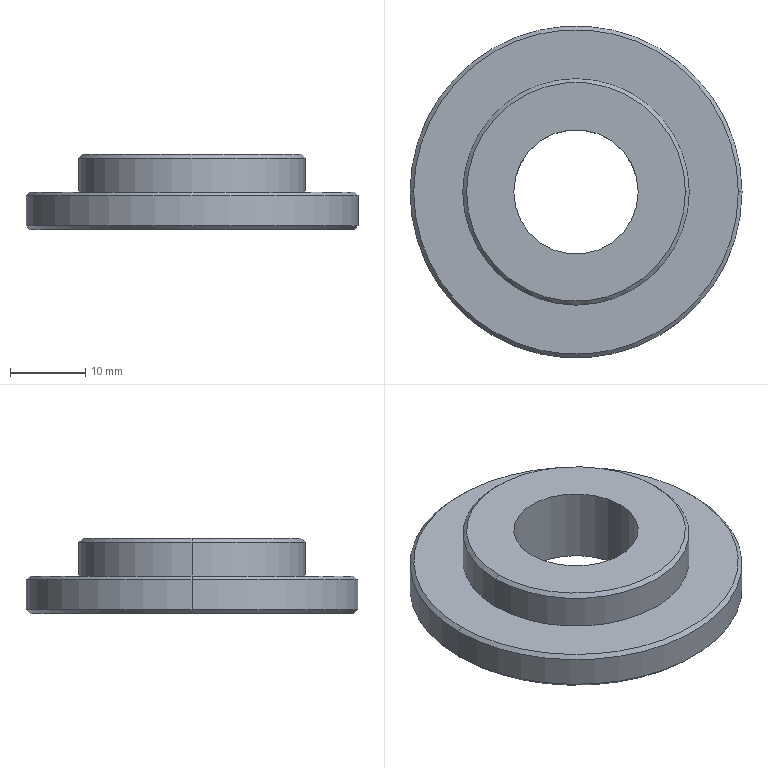Part | STEP file | 2025 Spring plate | 1 solid | 15 faces | box 44 x 44 x 10 mm | volume 8953 mm3 | cone 6 | cylinder 6 | plane 3 | commonest cylinder face diameters 16.5 x2 30 x2 44 x2
STEP:
#1=CARTESIAN_POINT('',(0.,0.,0.));
#2=DIRECTION('',(0.,0.,1.));
#3=DIRECTION('',(1.,0.,0.));
#4=AXIS2_PLACEMENT_3D('',#1,#2,#3);
#5=CARTESIAN_POINT('',(14.5,0.,10.));
#6=VERTEX_POINT('',#5);
#7=CARTESIAN_POINT('',(-14.5,0.,10.));
#8=VERTEX_POINT('',#7);
#9=CARTESIAN_POINT('',(0.,0.,10.));
#10=DIRECTION('',(0.,0.,1.));
#11=DIRECTION('',(1.,0.,0.));
#12=AXIS2_PLACEMENT_3D('',#9,#10,#11);
#13=CIRCLE('',#12,14.5);
#14=CARTESIAN_POINT('',(0.,0.,10.));
#15=DIRECTION('',(0.,0.,-1.));
#16=DIRECTION('',(-1.,0.,0.));
#17=AXIS2_PLACEMENT_3D('',#14,#15,#16);
#18=CONICAL_SURFACE('',#17,14.5,0.7854);
#19=CARTESIAN_POINT('',(3.142,0.));
#20=DIRECTION('',(-1.,0.));
#21=VECTOR('',#20,1.);
#22=LINE('',#19,#21);
#23=(GEOMETRIC_REPRESENTATION_CONTEXT(2)PARAMETRIC_REPRESENTATION_CONTEXT()REPRESENTATION_CONTEXT('',''));
#24=DEFINITIONAL_REPRESENTATION('',(#22),#23);
#25=PCURVE('',#18,#24);
#26=CARTESIAN_POINT('',(0.,0.,10.));
#27=DIRECTION('',(0.,0.,1.));
#28=DIRECTION('',(1.,0.,0.));
#29=AXIS2_PLACEMENT_3D('',#26,#27,#28);
#30=PLANE('',#29);
#31=CARTESIAN_POINT('',(0.,0.));
#32=DIRECTION('',(1.,0.));
#33=AXIS2_PLACEMENT_2D('',#31,#32);
#34=CIRCLE('',#33,14.5);
#35=(GEOMETRIC_REPRESENTATION_CONTEXT(2)PARAMETRIC_REPRESENTATION_CONTEXT()REPRESENTATION_CONTEXT('',''));
#36=DEFINITIONAL_REPRESENTATION('',(#34),#35);
#37=PCURVE('',#30,#36);
#38=SURFACE_CURVE('',#13,(#25,#37),.PCURVE_S1.);
#39=EDGE_CURVE('',#6,#8,#38,.T.);
#40=ORIENTED_EDGE('',*,*,#39,.F.);
#41=CARTESIAN_POINT('',(15.,0.,9.5));
#42=VERTEX_POINT('',#41);
#43=CARTESIAN_POINT('',(14.5,0.,10.));
#44=DIRECTION('',(0.7071,0.,-0.7071));
#45=VECTOR('',#44,1.);
#46=LINE('',#43,#45);
#47=CARTESIAN_POINT('',(3.142,0.));
#48=DIRECTION('',(0.,1.));
#49=VECTOR('',#48,1.);
#50=LINE('',#47,#49);
#51=(GEOMETRIC_REPRESENTATION_CONTEXT(2)PARAMETRIC_REPRESENTATION_CONTEXT()REPRESENTATION_CONTEXT('',''));
#52=DEFINITIONAL_REPRESENTATION('',(#50),#51);
#53=PCURVE('',#18,#52);
#54=CARTESIAN_POINT('',(0.,0.,10.));
#55=DIRECTION('',(0.,0.,-1.));
#56=DIRECTION('',(-1.,0.,0.));
#57=AXIS2_PLACEMENT_3D('',#54,#55,#56);
#58=CONICAL_SURFACE('',#57,14.5,0.7854);
#59=CARTESIAN_POINT('',(3.142,0.));
#60=DIRECTION('',(0.,1.));
#61=VECTOR('',#60,1.);
#62=LINE('',#59,#61);
#63=(GEOMETRIC_REPRESENTATION_CONTEXT(2)PARAMETRIC_REPRESENTATION_CONTEXT()REPRESENTATION_CONTEXT('',''));
#64=DEFINITIONAL_REPRESENTATION('',(#62),#63);
#65=PCURVE('',#58,#64);
#66=SURFACE_CURVE('',#46,(#53,#65),.PCURVE_S1.);
#67=EDGE_CURVE('',#6,#42,#66,.T.);
#68=ORIENTED_EDGE('',*,*,#67,.T.);
#69=CARTESIAN_POINT('',(-15.,0.,9.5));
#70=VERTEX_POINT('',#69);
#71=CARTESIAN_POINT('',(0.,0.,9.5));
#72=DIRECTION('',(0.,0.,-1.));
#73=DIRECTION('',(1.,0.,0.));
#74=AXIS2_PLACEMENT_3D('',#71,#72,#73);
#75=CIRCLE('',#74,15.);
#76=CARTESIAN_POINT('',(-3.142,0.5));
#77=DIRECTION('',(1.,0.));
#78=VECTOR('',#77,1.);
#79=LINE('',#76,#78);
#80=(GEOMETRIC_REPRESENTATION_CONTEXT(2)PARAMETRIC_REPRESENTATION_CONTEXT()REPRESENTATION_CONTEXT('',''));
#81=DEFINITIONAL_REPRESENTATION('',(#79),#80);
#82=PCURVE('',#18,#81);
#83=CARTESIAN_POINT('',(0.,0.,10.));
#84=DIRECTION('',(0.,0.,-1.));
#85=DIRECTION('',(-1.,0.,0.));
#86=AXIS2_PLACEMENT_3D('',#83,#84,#85);
#87=CYLINDRICAL_SURFACE('',#86,15.);
#88=CARTESIAN_POINT('',(-3.142,0.5));
#89=DIRECTION('',(1.,0.));
#90=VECTOR('',#89,1.);
#91=LINE('',#88,#90);
#92=(GEOMETRIC_REPRESENTATION_CONTEXT(2)PARAMETRIC_REPRESENTATION_CONTEXT()REPRESENTATION_CONTEXT('',''));
#93=DEFINITIONAL_REPRESENTATION('',(#91),#92);
#94=PCURVE('',#87,#93);
#95=SURFACE_CURVE('',#75,(#82,#94),.PCURVE_S1.);
#96=EDGE_CURVE('',#70,#42,#95,.T.);
#97=ORIENTED_EDGE('',*,*,#96,.F.);
#98=CARTESIAN_POINT('',(-14.5,0.,10.));
#99=DIRECTION('',(-0.7071,0.,-0.7071));
#100=VECTOR('',#99,1.);
#101=LINE('',#98,#100);
#102=CARTESIAN_POINT('',(0.,0.));
#103=DIRECTION('',(0.,1.));
#104=VECTOR('',#103,1.);
#105=LINE('',#102,#104);
#106=(GEOMETRIC_REPRESENTATION_CONTEXT(2)PARAMETRIC_REPRESENTATION_CONTEXT()REPRESENTATION_CONTEXT('',''));
#107=DEFINITIONAL_REPRESENTATION('',(#105),#106);
#108=PCURVE('',#18,#107);
#109=CARTESIAN_POINT('',(6.283,0.));
#110=DIRECTION('',(0.,1.));
#111=VECTOR('',#110,1.);
#112=LINE('',#109,#111);
#113=(GEOMETRIC_REPRESENTATION_CONTEXT(2)PARAMETRIC_REPRESENTATION_CONTEXT()REPRESENTATION_CONTEXT('',''));
#114=DEFINITIONAL_REPRESENTATION('',(#112),#113);
#115=PCURVE('',#58,#114);
#116=SURFACE_CURVE('',#101,(#108,#115),.PCURVE_S1.);
#117=EDGE_CURVE('',#8,#70,#116,.T.);
#118=ORIENTED_EDGE('',*,*,#117,.F.);
#119=EDGE_LOOP('',(#40,#68,#97,#118));
#120=FACE_BOUND('',#119,.T.);
#121=ADVANCED_FACE('',(#120),#18,.T.);
#122=CARTESIAN_POINT('',(21.5,0.,5.));
#123=VERTEX_POINT('',#122);
#124=CARTESIAN_POINT('',(-21.5,0.,5.));
#125=VERTEX_POINT('',#124);
#126=CARTESIAN_POINT('',(0.,0.,5.));
#127=DIRECTION('',(0.,0.,1.));
#128=DIRECTION('',(1.,0.,0.));
#129=AXIS2_PLACEMENT_3D('',#126,#127,#128);
#130=CIRCLE('',#129,21.5);
#131=CARTESIAN_POINT('',(0.,0.,5.));
#132=DIRECTION('',(0.,0.,-1.));
#133=DIRECTION('',(-1.,0.,0.));
#134=AXIS2_PLACEMENT_3D('',#131,#132,#133);
#135=CONICAL_SURFACE('',#134,21.5,0.7854);
#136=CARTESIAN_POINT('',(3.142,0.));
#137=DIRECTION('',(-1.,0.));
#138=VECTOR('',#137,1.);
#139=LINE('',#136,#138);
#140=(GEOMETRIC_REPRESENTATION_CONTEXT(2)PARAMETRIC_REPRESENTATION_CONTEXT()REPRESENTATION_CONTEXT('',''));
#141=DEFINITIONAL_REPRESENTATION('',(#139),#140);
#142=PCURVE('',#135,#141);
#143=CARTESIAN_POINT('',(0.,0.,5.));
#144=DIRECTION('',(0.,0.,1.));
#145=DIRECTION('',(1.,0.,0.));
#146=AXIS2_PLACEMENT_3D('',#143,#144,#145);
#147=PLANE('',#146);
#148=CARTESIAN_POINT('',(0.,0.));
#149=DIRECTION('',(1.,0.));
#150=AXIS2_PLACEMENT_2D('',#148,#149);
#151=CIRCLE('',#150,21.5);
#152=(GEOMETRIC_REPRESENTATION_CONTEXT(2)PARAMETRIC_REPRESENTATION_CONTEXT()REPRESENTATION_CONTEXT('',''));
#153=DEFINITIONAL_REPRESENTATION('',(#151),#152);
#154=PCURVE('',#147,#153);
#155=SURFACE_CURVE('',#130,(#142,#154),.PCURVE_S1.);
#156=EDGE_CURVE('',#123,#125,#155,.T.);
#157=ORIENTED_EDGE('',*,*,#156,.F.);
#158=CARTESIAN_POINT('',(22.,0.,4.5));
#159=VERTEX_POINT('',#158);
#160=CARTESIAN_POINT('',(21.5,0.,5.));
#161=DIRECTION('',(0.7071,0.,-0.7071));
#162=VECTOR('',#161,1.);
#163=LINE('',#160,#162);
#164=CARTESIAN_POINT('',(3.142,0.));
#165=DIRECTION('',(0.,1.));
#166=VECTOR('',#165,1.);
#167=LINE('',#164,#166);
#168=(GEOMETRIC_REPRESENTATION_CONTEXT(2)PARAMETRIC_REPRESENTATION_CONTEXT()REPRESENTATION_CONTEXT('',''));
#169=DEFINITIONAL_REPRESENTATION('',(#167),#168);
#170=PCURVE('',#135,#169);
#171=CARTESIAN_POINT('',(0.,0.,5.));
#172=DIRECTION('',(0.,0.,-1.));
#173=DIRECTION('',(-1.,0.,0.));
#174=AXIS2_PLACEMENT_3D('',#171,#172,#173);
#175=CONICAL_SURFACE('',#174,21.5,0.7854);
#176=CARTESIAN_POINT('',(3.142,0.));
#177=DIRECTION('',(0.,1.));
#178=VECTOR('',#177,1.);
#179=LINE('',#176,#178);
#180=(GEOMETRIC_REPRESENTATION_CONTEXT(2)PARAMETRIC_REPRESENTATION_CONTEXT()REPRESENTATION_CONTEXT('',''));
#181=DEFINITIONAL_REPRESENTATION('',(#179),#180);
#182=PCURVE('',#175,#181);
#183=SURFACE_CURVE('',#163,(#170,#182),.PCURVE_S1.);
#184=EDGE_CURVE('',#123,#159,#183,.T.);
#185=ORIENTED_EDGE('',*,*,#184,.T.);
#186=CARTESIAN_POINT('',(-22.,0.,4.5));
#187=VERTEX_POINT('',#186);
#188=CARTESIAN_POINT('',(0.,0.,4.5));
#189=DIRECTION('',(0.,0.,-1.));
#190=DIRECTION('',(1.,0.,0.));
#191=AXIS2_PLACEMENT_3D('',#188,#189,#190);
#192=CIRCLE('',#191,22.);
#193=CARTESIAN_POINT('',(-3.142,0.5));
#194=DIRECTION('',(1.,0.));
#195=VECTOR('',#194,1.);
#196=LINE('',#193,#195);
#197=(GEOMETRIC_REPRESENTATION_CONTEXT(2)PARAMETRIC_REPRESENTATION_CONTEXT()REPRESENTATION_CONTEXT('',''));
#198=DEFINITIONAL_REPRESENTATION('',(#196),#197);
#199=PCURVE('',#135,#198);
#200=CARTESIAN_POINT('',(0.,0.,5.));
#201=DIRECTION('',(0.,0.,-1.));
#202=DIRECTION('',(-1.,0.,0.));
#203=AXIS2_PLACEMENT_3D('',#200,#201,#202);
#204=CYLINDRICAL_SURFACE('',#203,22.);
#205=CARTESIAN_POINT('',(-3.142,0.5));
#206=DIRECTION('',(1.,0.));
#207=VECTOR('',#206,1.);
#208=LINE('',#205,#207);
#209=(GEOMETRIC_REPRESENTATION_CONTEXT(2)PARAMETRIC_REPRESENTATION_CONTEXT()REPRESENTATION_CONTEXT('',''));
#210=DEFINITIONAL_REPRESENTATION('',(#208),#209);
#211=PCURVE('',#204,#210);
#212=SURFACE_CURVE('',#192,(#199,#211),.PCURVE_S1.);
#213=EDGE_CURVE('',#187,#159,#212,.T.);
#214=ORIENTED_EDGE('',*,*,#213,.F.);
#215=CARTESIAN_POINT('',(-21.5,0.,5.));
#216=DIRECTION('',(-0.7071,0.,-0.7071));
#217=VECTOR('',#216,1.);
#218=LINE('',#215,#217);
#219=CARTESIAN_POINT('',(0.,0.));
#220=DIRECTION('',(0.,1.));
#221=VECTOR('',#220,1.);
#222=LINE('',#219,#221);
#223=(GEOMETRIC_REPRESENTATION_CONTEXT(2)PARAMETRIC_REPRESENTATION_CONTEXT()REPRESENTATION_CONTEXT('',''));
#224=DEFINITIONAL_REPRESENTATION('',(#222),#223);
#225=PCURVE('',#135,#224);
#226=CARTESIAN_POINT('',(6.283,0.));
#227=DIRECTION('',(0.,1.));
#228=VECTOR('',#227,1.);
#229=LINE('',#226,#228);
#230=(GEOMETRIC_REPRESENTATION_CONTEXT(2)PARAMETRIC_REPRESENTATION_CONTEXT()REPRESENTATION_CONTEXT('',''));
#231=DEFINITIONAL_REPRESENTATION('',(#229),#230);
#232=PCURVE('',#175,#231);
#233=SURFACE_CURVE('',#218,(#225,#232),.PCURVE_S1.);
#234=EDGE_CURVE('',#125,#187,#233,.T.);
#235=ORIENTED_EDGE('',*,*,#234,.F.);
#236=EDGE_LOOP('',(#157,#185,#214,#235));
#237=FACE_BOUND('',#236,.T.);
#238=ADVANCED_FACE('',(#237),#135,.T.);
#239=CARTESIAN_POINT('',(-21.5,0.,0.));
#240=VERTEX_POINT('',#239);
#241=CARTESIAN_POINT('',(21.5,0.,0.));
#242=VERTEX_POINT('',#241);
#243=CARTESIAN_POINT('',(0.,0.,0.));
#244=DIRECTION('',(0.,0.,-1.));
#245=DIRECTION('',(1.,0.,0.));
#246=AXIS2_PLACEMENT_3D('',#243,#244,#245);
#247=CIRCLE('',#246,21.5);
#248=CARTESIAN_POINT('',(0.,0.,0.5));
#249=DIRECTION('',(0.,0.,1.));
#250=DIRECTION('',(1.,0.,0.));
#251=AXIS2_PLACEMENT_3D('',#248,#249,#250);
#252=CONICAL_SURFACE('',#251,22.,0.7854);
#253=CARTESIAN_POINT('',(6.283,-0.5));
#254=DIRECTION('',(-1.,0.));
#255=VECTOR('',#254,1.);
#256=LINE('',#253,#255);
#257=(GEOMETRIC_REPRESENTATION_CONTEXT(2)PARAMETRIC_REPRESENTATION_CONTEXT()REPRESENTATION_CONTEXT('',''));
#258=DEFINITIONAL_REPRESENTATION('',(#256),#257);
#259=PCURVE('',#252,#258);
#260=CARTESIAN_POINT('',(0.,0.,0.));
#261=DIRECTION('',(0.,0.,1.));
#262=DIRECTION('',(1.,0.,0.));
#263=AXIS2_PLACEMENT_3D('',#260,#261,#262);
#264=PLANE('',#263);
#265=CARTESIAN_POINT('',(21.5,0.));
#266=CARTESIAN_POINT('',(21.5,-37.239));
#267=CARTESIAN_POINT('',(-10.75,-18.62));
#268=CARTESIAN_POINT('',(-43.,0.));
#269=CARTESIAN_POINT('',(-10.75,18.62));
#270=CARTESIAN_POINT('',(21.5,37.239));
#271=CARTESIAN_POINT('',(21.5,0.));
#272=(BOUNDED_CURVE()B_SPLINE_CURVE(2,(#265,#266,#267,#268,#269,#270,#271),.UNSPECIFIED.,.T.,.F.)B_SPLINE_CURVE_WITH_KNOTS((1,2,2,2,2,1),(-2.094,0.,2.094,4.189,6.283,8.378),.UNSPECIFIED.)CURVE()GEOMETRIC_REPRESENTATION_ITEM()RATIONAL_B_SPLINE_CURVE((1.,0.5,1.,0.5,1.,0.5,1.))REPRESENTATION_ITEM(''));
#273=(GEOMETRIC_REPRESENTATION_CONTEXT(2)PARAMETRIC_REPRESENTATION_CONTEXT()REPRESENTATION_CONTEXT('',''));
#274=DEFINITIONAL_REPRESENTATION('',(#272),#273);
#275=PCURVE('',#264,#274);
#276=SURFACE_CURVE('',#247,(#259,#275),.PCURVE_S1.);
#277=EDGE_CURVE('',#240,#242,#276,.T.);
#278=ORIENTED_EDGE('',*,*,#277,.F.);
#279=CARTESIAN_POINT('',(-22.,0.,0.5));
#280=VERTEX_POINT('',#279);
#281=CARTESIAN_POINT('',(-22.,0.,0.5));
#282=DIRECTION('',(-0.7071,0.,0.7071));
#283=VECTOR('',#282,1.);
#284=LINE('',#281,#283);
#285=CARTESIAN_POINT('',(3.142,0.));
#286=DIRECTION('',(0.,1.));
#287=VECTOR('',#286,1.);
#288=LINE('',#285,#287);
#289=(GEOMETRIC_REPRESENTATION_CONTEXT(2)PARAMETRIC_REPRESENTATION_CONTEXT()REPRESENTATION_CONTEXT('',''));
#290=DEFINITIONAL_REPRESENTATION('',(#288),#289);
#291=PCURVE('',#252,#290);
#292=CARTESIAN_POINT('',(0.,0.,0.5));
#293=DIRECTION('',(0.,0.,1.));
#294=DIRECTION('',(1.,0.,0.));
#295=AXIS2_PLACEMENT_3D('',#292,#293,#294);
#296=CONICAL_SURFACE('',#295,22.,0.7854);
#297=CARTESIAN_POINT('',(3.142,0.));
#298=DIRECTION('',(0.,1.));
#299=VECTOR('',#298,1.);
#300=LINE('',#297,#299);
#301=(GEOMETRIC_REPRESENTATION_CONTEXT(2)PARAMETRIC_REPRESENTATION_CONTEXT()REPRESENTATION_CONTEXT('',''));
#302=DEFINITIONAL_REPRESENTATION('',(#300),#301);
#303=PCURVE('',#296,#302);
#304=SURFACE_CURVE('',#284,(#291,#303),.PCURVE_S1.);
#305=EDGE_CURVE('',#240,#280,#304,.T.);
#306=ORIENTED_EDGE('',*,*,#305,.T.);
#307=CARTESIAN_POINT('',(22.,0.,0.5));
#308=VERTEX_POINT('',#307);
#309=CARTESIAN_POINT('',(0.,0.,0.5));
#310=DIRECTION('',(0.,0.,1.));
#311=DIRECTION('',(1.,0.,0.));
#312=AXIS2_PLACEMENT_3D('',#309,#310,#311);
#313=CIRCLE('',#312,22.);
#314=CARTESIAN_POINT('',(0.,0.));
#315=DIRECTION('',(1.,0.));
#316=VECTOR('',#315,1.);
#317=LINE('',#314,#316);
#318=(GEOMETRIC_REPRESENTATION_CONTEXT(2)PARAMETRIC_REPRESENTATION_CONTEXT()REPRESENTATION_CONTEXT('',''));
#319=DEFINITIONAL_REPRESENTATION('',(#317),#318);
#320=PCURVE('',#252,#319);
#321=CARTESIAN_POINT('',(3.142,4.5));
#322=DIRECTION('',(-1.,0.));
#323=VECTOR('',#322,1.);
#324=LINE('',#321,#323);
#325=(GEOMETRIC_REPRESENTATION_CONTEXT(2)PARAMETRIC_REPRESENTATION_CONTEXT()REPRESENTATION_CONTEXT('',''));
#326=DEFINITIONAL_REPRESENTATION('',(#324),#325);
#327=PCURVE('',#204,#326);
#328=SURFACE_CURVE('',#313,(#320,#327),.PCURVE_S1.);
#329=EDGE_CURVE('',#308,#280,#328,.T.);
#330=ORIENTED_EDGE('',*,*,#329,.F.);
#331=CARTESIAN_POINT('',(22.,0.,0.5));
#332=DIRECTION('',(0.7071,0.,0.7071));
#333=VECTOR('',#332,1.);
#334=LINE('',#331,#333);
#335=CARTESIAN_POINT('',(0.,0.));
#336=DIRECTION('',(0.,1.));
#337=VECTOR('',#336,1.);
#338=LINE('',#335,#337);
#339=(GEOMETRIC_REPRESENTATION_CONTEXT(2)PARAMETRIC_REPRESENTATION_CONTEXT()REPRESENTATION_CONTEXT('',''));
#340=DEFINITIONAL_REPRESENTATION('',(#338),#339);
#341=PCURVE('',#252,#340);
#342=CARTESIAN_POINT('',(6.283,0.));
#343=DIRECTION('',(0.,1.));
#344=VECTOR('',#343,1.);
#345=LINE('',#342,#344);
#346=(GEOMETRIC_REPRESENTATION_CONTEXT(2)PARAMETRIC_REPRESENTATION_CONTEXT()REPRESENTATION_CONTEXT('',''));
#347=DEFINITIONAL_REPRESENTATION('',(#345),#346);
#348=PCURVE('',#296,#347);
#349=SURFACE_CURVE('',#334,(#341,#348),.PCURVE_S1.);
#350=EDGE_CURVE('',#242,#308,#349,.T.);
#351=ORIENTED_EDGE('',*,*,#350,.F.);
#352=EDGE_LOOP('',(#278,#306,#330,#351));
#353=FACE_BOUND('',#352,.T.);
#354=ADVANCED_FACE('',(#353),#252,.T.);
#355=CARTESIAN_POINT('',(8.25,0.,0.));
#356=VERTEX_POINT('',#355);
#357=CARTESIAN_POINT('',(8.25,0.,10.));
#358=VERTEX_POINT('',#357);
#359=CARTESIAN_POINT('',(8.25,0.,0.));
#360=DIRECTION('',(0.,0.,1.));
#361=VECTOR('',#360,1.);
#362=LINE('',#359,#361);
#363=CARTESIAN_POINT('',(0.,0.,0.));
#364=DIRECTION('',(0.,0.,1.));
#365=DIRECTION('',(1.,0.,0.));
#366=AXIS2_PLACEMENT_3D('',#363,#364,#365);
#367=CYLINDRICAL_SURFACE('',#366,8.25);
#368=CARTESIAN_POINT('',(6.283,0.));
#369=DIRECTION('',(0.,1.));
#370=VECTOR('',#369,1.);
#371=LINE('',#368,#370);
#372=(GEOMETRIC_REPRESENTATION_CONTEXT(2)PARAMETRIC_REPRESENTATION_CONTEXT()REPRESENTATION_CONTEXT('',''));
#373=DEFINITIONAL_REPRESENTATION('',(#371),#372);
#374=PCURVE('',#367,#373);
#375=CARTESIAN_POINT('',(0.,0.,0.));
#376=DIRECTION('',(0.,0.,1.));
#377=DIRECTION('',(1.,0.,0.));
#378=AXIS2_PLACEMENT_3D('',#375,#376,#377);
#379=CYLINDRICAL_SURFACE('',#378,8.25);
#380=CARTESIAN_POINT('',(0.,0.));
#381=DIRECTION('',(0.,1.));
#382=VECTOR('',#381,1.);
#383=LINE('',#380,#382);
#384=(GEOMETRIC_REPRESENTATION_CONTEXT(2)PARAMETRIC_REPRESENTATION_CONTEXT()REPRESENTATION_CONTEXT('',''));
#385=DEFINITIONAL_REPRESENTATION('',(#383),#384);
#386=PCURVE('',#379,#385);
#387=SURFACE_CURVE('',#362,(#374,#386),.PCURVE_S1.);
#388=EDGE_CURVE('',#356,#358,#387,.T.);
#389=ORIENTED_EDGE('',*,*,#388,.T.);
#390=CARTESIAN_POINT('',(-8.25,0.,10.));
#391=VERTEX_POINT('',#390);
#392=CARTESIAN_POINT('',(0.,0.,10.));
#393=DIRECTION('',(0.,0.,1.));
#394=DIRECTION('',(1.,0.,0.));
#395=AXIS2_PLACEMENT_3D('',#392,#393,#394);
#396=CIRCLE('',#395,8.25);
#397=CARTESIAN_POINT('',(0.,10.));
#398=DIRECTION('',(1.,0.));
#399=VECTOR('',#398,1.);
#400=LINE('',#397,#399);
#401=(GEOMETRIC_REPRESENTATION_CONTEXT(2)PARAMETRIC_REPRESENTATION_CONTEXT()REPRESENTATION_CONTEXT('',''));
#402=DEFINITIONAL_REPRESENTATION('',(#400),#401);
#403=PCURVE('',#367,#402);
#404=CARTESIAN_POINT('',(0.,0.));
#405=DIRECTION('',(1.,0.));
#406=AXIS2_PLACEMENT_2D('',#404,#405);
#407=CIRCLE('',#406,8.25);
#408=(GEOMETRIC_REPRESENTATION_CONTEXT(2)PARAMETRIC_REPRESENTATION_CONTEXT()REPRESENTATION_CONTEXT('',''));
#409=DEFINITIONAL_REPRESENTATION('',(#407),#408);
#410=PCURVE('',#30,#409);
#411=SURFACE_CURVE('',#396,(#403,#410),.PCURVE_S1.);
#412=EDGE_CURVE('',#391,#358,#411,.T.);
#413=ORIENTED_EDGE('',*,*,#412,.F.);
#414=CARTESIAN_POINT('',(-8.25,0.,0.));
#415=VERTEX_POINT('',#414);
#416=CARTESIAN_POINT('',(-8.25,0.,0.));
#417=DIRECTION('',(0.,0.,1.));
#418=VECTOR('',#417,1.);
#419=LINE('',#416,#418);
#420=CARTESIAN_POINT('',(3.142,0.));
#421=DIRECTION('',(0.,1.));
#422=VECTOR('',#421,1.);
#423=LINE('',#420,#422);
#424=(GEOMETRIC_REPRESENTATION_CONTEXT(2)PARAMETRIC_REPRESENTATION_CONTEXT()REPRESENTATION_CONTEXT('',''));
#425=DEFINITIONAL_REPRESENTATION('',(#423),#424);
#426=PCURVE('',#367,#425);
#427=CARTESIAN_POINT('',(3.142,0.));
#428=DIRECTION('',(0.,1.));
#429=VECTOR('',#428,1.);
#430=LINE('',#427,#429);
#431=(GEOMETRIC_REPRESENTATION_CONTEXT(2)PARAMETRIC_REPRESENTATION_CONTEXT()REPRESENTATION_CONTEXT('',''));
#432=DEFINITIONAL_REPRESENTATION('',(#430),#431);
#433=PCURVE('',#379,#432);
#434=SURFACE_CURVE('',#419,(#426,#433),.PCURVE_S1.);
#435=EDGE_CURVE('',#415,#391,#434,.T.);
#436=ORIENTED_EDGE('',*,*,#435,.F.);
#437=CARTESIAN_POINT('',(0.,0.,0.));
#438=DIRECTION('',(0.,0.,1.));
#439=DIRECTION('',(1.,0.,0.));
#440=AXIS2_PLACEMENT_3D('',#437,#438,#439);
#441=CIRCLE('',#440,8.25);
#442=CARTESIAN_POINT('',(0.,0.));
#443=DIRECTION('',(1.,0.));
#444=VECTOR('',#443,1.);
#445=LINE('',#442,#444);
#446=(GEOMETRIC_REPRESENTATION_CONTEXT(2)PARAMETRIC_REPRESENTATION_CONTEXT()REPRESENTATION_CONTEXT('',''));
#447=DEFINITIONAL_REPRESENTATION('',(#445),#446);
#448=PCURVE('',#367,#447);
#449=CARTESIAN_POINT('',(0.,0.));
#450=DIRECTION('',(1.,0.));
#451=AXIS2_PLACEMENT_2D('',#449,#450);
#452=CIRCLE('',#451,8.25);
#453=(GEOMETRIC_REPRESENTATION_CONTEXT(2)PARAMETRIC_REPRESENTATION_CONTEXT()REPRESENTATION_CONTEXT('',''));
#454=DEFINITIONAL_REPRESENTATION('',(#452),#453);
#455=PCURVE('',#264,#454);
#456=SURFACE_CURVE('',#441,(#448,#455),.PCURVE_S1.);
#457=EDGE_CURVE('',#415,#356,#456,.T.);
#458=ORIENTED_EDGE('',*,*,#457,.T.);
#459=EDGE_LOOP('',(#389,#413,#436,#458));
#460=FACE_BOUND('',#459,.F.);
#461=ADVANCED_FACE('',(#460),#367,.F.);
#462=ORIENTED_EDGE('',*,*,#96,.T.);
#463=CARTESIAN_POINT('',(15.,0.,5.));
#464=VERTEX_POINT('',#463);
#465=CARTESIAN_POINT('',(15.,0.,10.));
#466=DIRECTION('',(0.,0.,-1.));
#467=VECTOR('',#466,1.);
#468=LINE('',#465,#467);
#469=CARTESIAN_POINT('',(3.142,0.));
#470=DIRECTION('',(0.,1.));
#471=VECTOR('',#470,1.);
#472=LINE('',#469,#471);
#473=(GEOMETRIC_REPRESENTATION_CONTEXT(2)PARAMETRIC_REPRESENTATION_CONTEXT()REPRESENTATION_CONTEXT('',''));
#474=DEFINITIONAL_REPRESENTATION('',(#472),#473);
#475=PCURVE('',#87,#474);
#476=CARTESIAN_POINT('',(0.,0.,10.));
#477=DIRECTION('',(0.,0.,-1.));
#478=DIRECTION('',(-1.,0.,0.));
#479=AXIS2_PLACEMENT_3D('',#476,#477,#478);
#480=CYLINDRICAL_SURFACE('',#479,15.);
#481=CARTESIAN_POINT('',(3.142,0.));
#482=DIRECTION('',(0.,1.));
#483=VECTOR('',#482,1.);
#484=LINE('',#481,#483);
#485=(GEOMETRIC_REPRESENTATION_CONTEXT(2)PARAMETRIC_REPRESENTATION_CONTEXT()REPRESENTATION_CONTEXT('',''));
#486=DEFINITIONAL_REPRESENTATION('',(#484),#485);
#487=PCURVE('',#480,#486);
#488=SURFACE_CURVE('',#468,(#475,#487),.PCURVE_S1.);
#489=EDGE_CURVE('',#42,#464,#488,.T.);
#490=ORIENTED_EDGE('',*,*,#489,.T.);
#491=CARTESIAN_POINT('',(-15.,0.,5.));
#492=VERTEX_POINT('',#491);
#493=CARTESIAN_POINT('',(0.,0.,5.));
#494=DIRECTION('',(0.,0.,1.));
#495=DIRECTION('',(1.,0.,0.));
#496=AXIS2_PLACEMENT_3D('',#493,#494,#495);
#497=CIRCLE('',#496,15.);
#498=CARTESIAN_POINT('',(3.142,5.));
#499=DIRECTION('',(-1.,0.));
#500=VECTOR('',#499,1.);
#501=LINE('',#498,#500);
#502=(GEOMETRIC_REPRESENTATION_CONTEXT(2)PARAMETRIC_REPRESENTATION_CONTEXT()REPRESENTATION_CONTEXT('',''));
#503=DEFINITIONAL_REPRESENTATION('',(#501),#502);
#504=PCURVE('',#87,#503);
#505=CARTESIAN_POINT('',(0.,0.));
#506=DIRECTION('',(1.,0.));
#507=AXIS2_PLACEMENT_2D('',#505,#506);
#508=CIRCLE('',#507,15.);
#509=(GEOMETRIC_REPRESENTATION_CONTEXT(2)PARAMETRIC_REPRESENTATION_CONTEXT()REPRESENTATION_CONTEXT('',''));
#510=DEFINITIONAL_REPRESENTATION('',(#508),#509);
#511=PCURVE('',#147,#510);
#512=SURFACE_CURVE('',#497,(#504,#511),.PCURVE_S1.);
#513=EDGE_CURVE('',#464,#492,#512,.T.);
#514=ORIENTED_EDGE('',*,*,#513,.T.);
#515=CARTESIAN_POINT('',(-15.,0.,10.));
#516=DIRECTION('',(0.,0.,-1.));
#517=VECTOR('',#516,1.);
#518=LINE('',#515,#517);
#519=CARTESIAN_POINT('',(0.,0.));
#520=DIRECTION('',(0.,1.));
#521=VECTOR('',#520,1.);
#522=LINE('',#519,#521);
#523=(GEOMETRIC_REPRESENTATION_CONTEXT(2)PARAMETRIC_REPRESENTATION_CONTEXT()REPRESENTATION_CONTEXT('',''));
#524=DEFINITIONAL_REPRESENTATION('',(#522),#523);
#525=PCURVE('',#87,#524);
#526=CARTESIAN_POINT('',(6.283,0.));
#527=DIRECTION('',(0.,1.));
#528=VECTOR('',#527,1.);
#529=LINE('',#526,#528);
#530=(GEOMETRIC_REPRESENTATION_CONTEXT(2)PARAMETRIC_REPRESENTATION_CONTEXT()REPRESENTATION_CONTEXT('',''));
#531=DEFINITIONAL_REPRESENTATION('',(#529),#530);
#532=PCURVE('',#480,#531);
#533=SURFACE_CURVE('',#518,(#525,#532),.PCURVE_S1.);
#534=EDGE_CURVE('',#70,#492,#533,.T.);
#535=ORIENTED_EDGE('',*,*,#534,.F.);
#536=EDGE_LOOP('',(#462,#490,#514,#535));
#537=FACE_BOUND('',#536,.T.);
#538=ADVANCED_FACE('',(#537),#87,.T.);
#539=ORIENTED_EDGE('',*,*,#213,.T.);
#540=CARTESIAN_POINT('',(22.,0.,5.));
#541=DIRECTION('',(0.,0.,-1.));
#542=VECTOR('',#541,1.);
#543=LINE('',#540,#542);
#544=CARTESIAN_POINT('',(3.142,0.));
#545=DIRECTION('',(0.,1.));
#546=VECTOR('',#545,1.);
#547=LINE('',#544,#546);
#548=(GEOMETRIC_REPRESENTATION_CONTEXT(2)PARAMETRIC_REPRESENTATION_CONTEXT()REPRESENTATION_CONTEXT('',''));
#549=DEFINITIONAL_REPRESENTATION('',(#547),#548);
#550=PCURVE('',#204,#549);
#551=CARTESIAN_POINT('',(0.,0.,5.));
#552=DIRECTION('',(0.,0.,-1.));
#553=DIRECTION('',(-1.,0.,0.));
#554=AXIS2_PLACEMENT_3D('',#551,#552,#553);
#555=CYLINDRICAL_SURFACE('',#554,22.);
#556=CARTESIAN_POINT('',(3.142,0.));
#557=DIRECTION('',(0.,1.));
#558=VECTOR('',#557,1.);
#559=LINE('',#556,#558);
#560=(GEOMETRIC_REPRESENTATION_CONTEXT(2)PARAMETRIC_REPRESENTATION_CONTEXT()REPRESENTATION_CONTEXT('',''));
#561=DEFINITIONAL_REPRESENTATION('',(#559),#560);
#562=PCURVE('',#555,#561);
#563=SURFACE_CURVE('',#543,(#550,#562),.PCURVE_S1.);
#564=EDGE_CURVE('',#159,#308,#563,.T.);
#565=ORIENTED_EDGE('',*,*,#564,.T.);
#566=ORIENTED_EDGE('',*,*,#329,.T.);
#567=CARTESIAN_POINT('',(-22.,0.,5.));
#568=DIRECTION('',(0.,0.,-1.));
#569=VECTOR('',#568,1.);
#570=LINE('',#567,#569);
#571=CARTESIAN_POINT('',(0.,0.));
#572=DIRECTION('',(0.,1.));
#573=VECTOR('',#572,1.);
#574=LINE('',#571,#573);
#575=(GEOMETRIC_REPRESENTATION_CONTEXT(2)PARAMETRIC_REPRESENTATION_CONTEXT()REPRESENTATION_CONTEXT('',''));
#576=DEFINITIONAL_REPRESENTATION('',(#574),#575);
#577=PCURVE('',#204,#576);
#578=CARTESIAN_POINT('',(6.283,0.));
#579=DIRECTION('',(0.,1.));
#580=VECTOR('',#579,1.);
#581=LINE('',#578,#580);
#582=(GEOMETRIC_REPRESENTATION_CONTEXT(2)PARAMETRIC_REPRESENTATION_CONTEXT()REPRESENTATION_CONTEXT('',''));
#583=DEFINITIONAL_REPRESENTATION('',(#581),#582);
#584=PCURVE('',#555,#583);
#585=SURFACE_CURVE('',#570,(#577,#584),.PCURVE_S1.);
#586=EDGE_CURVE('',#187,#280,#585,.T.);
#587=ORIENTED_EDGE('',*,*,#586,.F.);
#588=EDGE_LOOP('',(#539,#565,#566,#587));
#589=FACE_BOUND('',#588,.T.);
#590=ADVANCED_FACE('',(#589),#204,.T.);
#591=CARTESIAN_POINT('',(0.,0.,5.));
#592=DIRECTION('',(0.,0.,1.));
#593=DIRECTION('',(1.,0.,0.));
#594=AXIS2_PLACEMENT_3D('',#591,#592,#593);
#595=CIRCLE('',#594,21.5);
#596=CARTESIAN_POINT('',(0.,0.));
#597=DIRECTION('',(1.,0.));
#598=AXIS2_PLACEMENT_2D('',#596,#597);
#599=CIRCLE('',#598,21.5);
#600=(GEOMETRIC_REPRESENTATION_CONTEXT(2)PARAMETRIC_REPRESENTATION_CONTEXT()REPRESENTATION_CONTEXT('',''));
#601=DEFINITIONAL_REPRESENTATION('',(#599),#600);
#602=PCURVE('',#147,#601);
#603=CARTESIAN_POINT('',(9.425,0.));
#604=DIRECTION('',(-1.,0.));
#605=VECTOR('',#604,1.);
#606=LINE('',#603,#605);
#607=(GEOMETRIC_REPRESENTATION_CONTEXT(2)PARAMETRIC_REPRESENTATION_CONTEXT()REPRESENTATION_CONTEXT('',''));
#608=DEFINITIONAL_REPRESENTATION('',(#606),#607);
#609=PCURVE('',#175,#608);
#610=SURFACE_CURVE('',#595,(#602,#609),.PCURVE_S1.);
#611=EDGE_CURVE('',#125,#123,#610,.T.);
#612=ORIENTED_EDGE('',*,*,#611,.T.);
#613=ORIENTED_EDGE('',*,*,#156,.T.);
#614=EDGE_LOOP('',(#612,#613));
#615=FACE_BOUND('',#614,.T.);
#616=CARTESIAN_POINT('',(0.,0.,5.));
#617=DIRECTION('',(0.,0.,1.));
#618=DIRECTION('',(1.,0.,0.));
#619=AXIS2_PLACEMENT_3D('',#616,#617,#618);
#620=CIRCLE('',#619,15.);
#621=CARTESIAN_POINT('',(0.,0.));
#622=DIRECTION('',(1.,0.));
#623=AXIS2_PLACEMENT_2D('',#621,#622);
#624=CIRCLE('',#623,15.);
#625=(GEOMETRIC_REPRESENTATION_CONTEXT(2)PARAMETRIC_REPRESENTATION_CONTEXT()REPRESENTATION_CONTEXT('',''));
#626=DEFINITIONAL_REPRESENTATION('',(#624),#625);
#627=PCURVE('',#147,#626);
#628=CARTESIAN_POINT('',(9.425,5.));
#629=DIRECTION('',(-1.,0.));
#630=VECTOR('',#629,1.);
#631=LINE('',#628,#630);
#632=(GEOMETRIC_REPRESENTATION_CONTEXT(2)PARAMETRIC_REPRESENTATION_CONTEXT()REPRESENTATION_CONTEXT('',''));
#633=DEFINITIONAL_REPRESENTATION('',(#631),#632);
#634=PCURVE('',#480,#633);
#635=SURFACE_CURVE('',#620,(#627,#634),.PCURVE_S1.);
#636=EDGE_CURVE('',#492,#464,#635,.T.);
#637=ORIENTED_EDGE('',*,*,#636,.F.);
#638=ORIENTED_EDGE('',*,*,#513,.F.);
#639=EDGE_LOOP('',(#637,#638));
#640=FACE_BOUND('',#639,.T.);
#641=ADVANCED_FACE('',(#615,#640),#147,.T.);
#642=ORIENTED_EDGE('',*,*,#564,.F.);
#643=CARTESIAN_POINT('',(0.,0.,4.5));
#644=DIRECTION('',(0.,0.,-1.));
#645=DIRECTION('',(1.,0.,0.));
#646=AXIS2_PLACEMENT_3D('',#643,#644,#645);
#647=CIRCLE('',#646,22.);
#648=CARTESIAN_POINT('',(3.142,0.5));
#649=DIRECTION('',(1.,0.));
#650=VECTOR('',#649,1.);
#651=LINE('',#648,#650);
#652=(GEOMETRIC_REPRESENTATION_CONTEXT(2)PARAMETRIC_REPRESENTATION_CONTEXT()REPRESENTATION_CONTEXT('',''));
#653=DEFINITIONAL_REPRESENTATION('',(#651),#652);
#654=PCURVE('',#555,#653);
#655=CARTESIAN_POINT('',(3.142,0.5));
#656=DIRECTION('',(1.,0.));
#657=VECTOR('',#656,1.);
#658=LINE('',#655,#657);
#659=(GEOMETRIC_REPRESENTATION_CONTEXT(2)PARAMETRIC_REPRESENTATION_CONTEXT()REPRESENTATION_CONTEXT('',''));
#660=DEFINITIONAL_REPRESENTATION('',(#658),#659);
#661=PCURVE('',#175,#660);
#662=SURFACE_CURVE('',#647,(#654,#661),.PCURVE_S1.);
#663=EDGE_CURVE('',#159,#187,#662,.T.);
#664=ORIENTED_EDGE('',*,*,#663,.T.);
#665=ORIENTED_EDGE('',*,*,#586,.T.);
#666=CARTESIAN_POINT('',(0.,0.,0.5));
#667=DIRECTION('',(0.,0.,1.));
#668=DIRECTION('',(1.,0.,0.));
#669=AXIS2_PLACEMENT_3D('',#666,#667,#668);
#670=CIRCLE('',#669,22.);
#671=CARTESIAN_POINT('',(9.425,4.5));
#672=DIRECTION('',(-1.,0.));
#673=VECTOR('',#672,1.);
#674=LINE('',#671,#673);
#675=(GEOMETRIC_REPRESENTATION_CONTEXT(2)PARAMETRIC_REPRESENTATION_CONTEXT()REPRESENTATION_CONTEXT('',''));
#676=DEFINITIONAL_REPRESENTATION('',(#674),#675);
#677=PCURVE('',#555,#676);
#678=CARTESIAN_POINT('',(0.,0.));
#679=DIRECTION('',(1.,0.));
#680=VECTOR('',#679,1.);
#681=LINE('',#678,#680);
#682=(GEOMETRIC_REPRESENTATION_CONTEXT(2)PARAMETRIC_REPRESENTATION_CONTEXT()REPRESENTATION_CONTEXT('',''));
#683=DEFINITIONAL_REPRESENTATION('',(#681),#682);
#684=PCURVE('',#296,#683);
#685=SURFACE_CURVE('',#670,(#677,#684),.PCURVE_S1.);
#686=EDGE_CURVE('',#280,#308,#685,.T.);
#687=ORIENTED_EDGE('',*,*,#686,.T.);
#688=EDGE_LOOP('',(#642,#664,#665,#687));
#689=FACE_BOUND('',#688,.T.);
#690=ADVANCED_FACE('',(#689),#555,.T.);
#691=CARTESIAN_POINT('',(0.,0.,0.));
#692=DIRECTION('',(0.,0.,-1.));
#693=DIRECTION('',(1.,0.,0.));
#694=AXIS2_PLACEMENT_3D('',#691,#692,#693);
#695=CIRCLE('',#694,21.5);
#696=CARTESIAN_POINT('',(21.5,0.));
#697=CARTESIAN_POINT('',(21.5,-37.239));
#698=CARTESIAN_POINT('',(-10.75,-18.62));
#699=CARTESIAN_POINT('',(-43.,0.));
#700=CARTESIAN_POINT('',(-10.75,18.62));
#701=CARTESIAN_POINT('',(21.5,37.239));
#702=CARTESIAN_POINT('',(21.5,0.));
#703=(BOUNDED_CURVE()B_SPLINE_CURVE(2,(#696,#697,#698,#699,#700,#701,#702),.UNSPECIFIED.,.T.,.F.)B_SPLINE_CURVE_WITH_KNOTS((1,2,2,2,2,1),(-2.094,0.,2.094,4.189,6.283,8.378),.UNSPECIFIED.)CURVE()GEOMETRIC_REPRESENTATION_ITEM()RATIONAL_B_SPLINE_CURVE((1.,0.5,1.,0.5,1.,0.5,1.))REPRESENTATION_ITEM(''));
#704=(GEOMETRIC_REPRESENTATION_CONTEXT(2)PARAMETRIC_REPRESENTATION_CONTEXT()REPRESENTATION_CONTEXT('',''));
#705=DEFINITIONAL_REPRESENTATION('',(#703),#704);
#706=PCURVE('',#264,#705);
#707=CARTESIAN_POINT('',(6.283,-0.5));
#708=DIRECTION('',(-1.,0.));
#709=VECTOR('',#708,1.);
#710=LINE('',#707,#709);
#711=(GEOMETRIC_REPRESENTATION_CONTEXT(2)PARAMETRIC_REPRESENTATION_CONTEXT()REPRESENTATION_CONTEXT('',''));
#712=DEFINITIONAL_REPRESENTATION('',(#710),#711);
#713=PCURVE('',#296,#712);
#714=SURFACE_CURVE('',#695,(#706,#713),.PCURVE_S1.);
#715=EDGE_CURVE('',#242,#240,#714,.T.);
#716=ORIENTED_EDGE('',*,*,#715,.T.);
#717=ORIENTED_EDGE('',*,*,#277,.T.);
#718=EDGE_LOOP('',(#716,#717));
#719=FACE_BOUND('',#718,.T.);
#720=CARTESIAN_POINT('',(0.,0.,0.));
#721=DIRECTION('',(0.,0.,1.));
#722=DIRECTION('',(1.,0.,0.));
#723=AXIS2_PLACEMENT_3D('',#720,#721,#722);
#724=CIRCLE('',#723,8.25);
#725=CARTESIAN_POINT('',(0.,0.));
#726=DIRECTION('',(1.,0.));
#727=AXIS2_PLACEMENT_2D('',#725,#726);
#728=CIRCLE('',#727,8.25);
#729=(GEOMETRIC_REPRESENTATION_CONTEXT(2)PARAMETRIC_REPRESENTATION_CONTEXT()REPRESENTATION_CONTEXT('',''));
#730=DEFINITIONAL_REPRESENTATION('',(#728),#729);
#731=PCURVE('',#264,#730);
#732=CARTESIAN_POINT('',(0.,0.));
#733=DIRECTION('',(1.,0.));
#734=VECTOR('',#733,1.);
#735=LINE('',#732,#734);
#736=(GEOMETRIC_REPRESENTATION_CONTEXT(2)PARAMETRIC_REPRESENTATION_CONTEXT()REPRESENTATION_CONTEXT('',''));
#737=DEFINITIONAL_REPRESENTATION('',(#735),#736);
#738=PCURVE('',#379,#737);
#739=SURFACE_CURVE('',#724,(#731,#738),.PCURVE_S1.);
#740=EDGE_CURVE('',#356,#415,#739,.T.);
#741=ORIENTED_EDGE('',*,*,#740,.T.);
#742=ORIENTED_EDGE('',*,*,#457,.T.);
#743=EDGE_LOOP('',(#741,#742));
#744=FACE_BOUND('',#743,.T.);
#745=ADVANCED_FACE('',(#719,#744),#264,.F.);
#746=ORIENTED_EDGE('',*,*,#489,.F.);
#747=CARTESIAN_POINT('',(0.,0.,9.5));
#748=DIRECTION('',(0.,0.,-1.));
#749=DIRECTION('',(1.,0.,0.));
#750=AXIS2_PLACEMENT_3D('',#747,#748,#749);
#751=CIRCLE('',#750,15.);
#752=CARTESIAN_POINT('',(3.142,0.5));
#753=DIRECTION('',(1.,0.));
#754=VECTOR('',#753,1.);
#755=LINE('',#752,#754);
#756=(GEOMETRIC_REPRESENTATION_CONTEXT(2)PARAMETRIC_REPRESENTATION_CONTEXT()REPRESENTATION_CONTEXT('',''));
#757=DEFINITIONAL_REPRESENTATION('',(#755),#756);
#758=PCURVE('',#480,#757);
#759=CARTESIAN_POINT('',(3.142,0.5));
#760=DIRECTION('',(1.,0.));
#761=VECTOR('',#760,1.);
#762=LINE('',#759,#761);
#763=(GEOMETRIC_REPRESENTATION_CONTEXT(2)PARAMETRIC_REPRESENTATION_CONTEXT()REPRESENTATION_CONTEXT('',''));
#764=DEFINITIONAL_REPRESENTATION('',(#762),#763);
#765=PCURVE('',#58,#764);
#766=SURFACE_CURVE('',#751,(#758,#765),.PCURVE_S1.);
#767=EDGE_CURVE('',#42,#70,#766,.T.);
#768=ORIENTED_EDGE('',*,*,#767,.T.);
#769=ORIENTED_EDGE('',*,*,#534,.T.);
#770=ORIENTED_EDGE('',*,*,#636,.T.);
#771=EDGE_LOOP('',(#746,#768,#769,#770));
#772=FACE_BOUND('',#771,.T.);
#773=ADVANCED_FACE('',(#772),#480,.T.);
#774=CARTESIAN_POINT('',(0.,0.,10.));
#775=DIRECTION('',(0.,0.,1.));
#776=DIRECTION('',(1.,0.,0.));
#777=AXIS2_PLACEMENT_3D('',#774,#775,#776);
#778=CIRCLE('',#777,14.5);
#779=CARTESIAN_POINT('',(0.,0.));
#780=DIRECTION('',(1.,0.));
#781=AXIS2_PLACEMENT_2D('',#779,#780);
#782=CIRCLE('',#781,14.5);
#783=(GEOMETRIC_REPRESENTATION_CONTEXT(2)PARAMETRIC_REPRESENTATION_CONTEXT()REPRESENTATION_CONTEXT('',''));
#784=DEFINITIONAL_REPRESENTATION('',(#782),#783);
#785=PCURVE('',#30,#784);
#786=CARTESIAN_POINT('',(9.425,0.));
#787=DIRECTION('',(-1.,0.));
#788=VECTOR('',#787,1.);
#789=LINE('',#786,#788);
#790=(GEOMETRIC_REPRESENTATION_CONTEXT(2)PARAMETRIC_REPRESENTATION_CONTEXT()REPRESENTATION_CONTEXT('',''));
#791=DEFINITIONAL_REPRESENTATION('',(#789),#790);
#792=PCURVE('',#58,#791);
#793=SURFACE_CURVE('',#778,(#785,#792),.PCURVE_S1.);
#794=EDGE_CURVE('',#8,#6,#793,.T.);
#795=ORIENTED_EDGE('',*,*,#794,.T.);
#796=ORIENTED_EDGE('',*,*,#39,.T.);
#797=EDGE_LOOP('',(#795,#796));
#798=FACE_BOUND('',#797,.T.);
#799=CARTESIAN_POINT('',(0.,0.,10.));
#800=DIRECTION('',(0.,0.,1.));
#801=DIRECTION('',(1.,0.,0.));
#802=AXIS2_PLACEMENT_3D('',#799,#800,#801);
#803=CIRCLE('',#802,8.25);
#804=CARTESIAN_POINT('',(0.,0.));
#805=DIRECTION('',(1.,0.));
#806=AXIS2_PLACEMENT_2D('',#804,#805);
#807=CIRCLE('',#806,8.25);
#808=(GEOMETRIC_REPRESENTATION_CONTEXT(2)PARAMETRIC_REPRESENTATION_CONTEXT()REPRESENTATION_CONTEXT('',''));
#809=DEFINITIONAL_REPRESENTATION('',(#807),#808);
#810=PCURVE('',#30,#809);
#811=CARTESIAN_POINT('',(0.,10.));
#812=DIRECTION('',(1.,0.));
#813=VECTOR('',#812,1.);
#814=LINE('',#811,#813);
#815=(GEOMETRIC_REPRESENTATION_CONTEXT(2)PARAMETRIC_REPRESENTATION_CONTEXT()REPRESENTATION_CONTEXT('',''));
#816=DEFINITIONAL_REPRESENTATION('',(#814),#815);
#817=PCURVE('',#379,#816);
#818=SURFACE_CURVE('',#803,(#810,#817),.PCURVE_S1.);
#819=EDGE_CURVE('',#358,#391,#818,.T.);
#820=ORIENTED_EDGE('',*,*,#819,.F.);
#821=ORIENTED_EDGE('',*,*,#412,.F.);
#822=EDGE_LOOP('',(#820,#821));
#823=FACE_BOUND('',#822,.T.);
#824=ADVANCED_FACE('',(#798,#823),#30,.T.);
#825=ORIENTED_EDGE('',*,*,#819,.F.);
#826=ORIENTED_EDGE('',*,*,#388,.F.);
#827=ORIENTED_EDGE('',*,*,#740,.T.);
#828=ORIENTED_EDGE('',*,*,#435,.T.);
#829=EDGE_LOOP('',(#825,#826,#827,#828));
#830=FACE_BOUND('',#829,.F.);
#831=ADVANCED_FACE('',(#830),#379,.F.);
#832=ORIENTED_EDGE('',*,*,#305,.F.);
#833=ORIENTED_EDGE('',*,*,#715,.F.);
#834=ORIENTED_EDGE('',*,*,#350,.T.);
#835=ORIENTED_EDGE('',*,*,#686,.F.);
#836=EDGE_LOOP('',(#832,#833,#834,#835));
#837=FACE_BOUND('',#836,.T.);
#838=ADVANCED_FACE('',(#837),#296,.T.);
#839=ORIENTED_EDGE('',*,*,#184,.F.);
#840=ORIENTED_EDGE('',*,*,#611,.F.);
#841=ORIENTED_EDGE('',*,*,#234,.T.);
#842=ORIENTED_EDGE('',*,*,#663,.F.);
#843=EDGE_LOOP('',(#839,#840,#841,#842));
#844=FACE_BOUND('',#843,.T.);
#845=ADVANCED_FACE('',(#844),#175,.T.);
#846=ORIENTED_EDGE('',*,*,#67,.F.);
#847=ORIENTED_EDGE('',*,*,#794,.F.);
#848=ORIENTED_EDGE('',*,*,#117,.T.);
#849=ORIENTED_EDGE('',*,*,#767,.F.);
#850=EDGE_LOOP('',(#846,#847,#848,#849));
#851=FACE_BOUND('',#850,.T.);
#852=ADVANCED_FACE('',(#851),#58,.T.);
#853=CLOSED_SHELL('',(#121,#238,#354,#461,#538,#590,#641,#690,#745,#773,#824,#831,#838,#845,#852));
#854=MANIFOLD_SOLID_BREP('',#853);
#855=(LENGTH_UNIT()NAMED_UNIT(*)SI_UNIT(.MILLI.,.METRE.));
#856=UNCERTAINTY_MEASURE_WITH_UNIT(LENGTH_MEASURE(0.0000001),#855,'','');
#857=(NAMED_UNIT(*)PLANE_ANGLE_UNIT()SI_UNIT($,.RADIAN.));
#858=(NAMED_UNIT(*)SI_UNIT($,.STERADIAN.)SOLID_ANGLE_UNIT());
#859=(GEOMETRIC_REPRESENTATION_CONTEXT(3)GLOBAL_UNCERTAINTY_ASSIGNED_CONTEXT((#856))GLOBAL_UNIT_ASSIGNED_CONTEXT((#855,#857,#858))REPRESENTATION_CONTEXT('',''));
#860=ADVANCED_BREP_SHAPE_REPRESENTATION('',(#4,#854),#859);